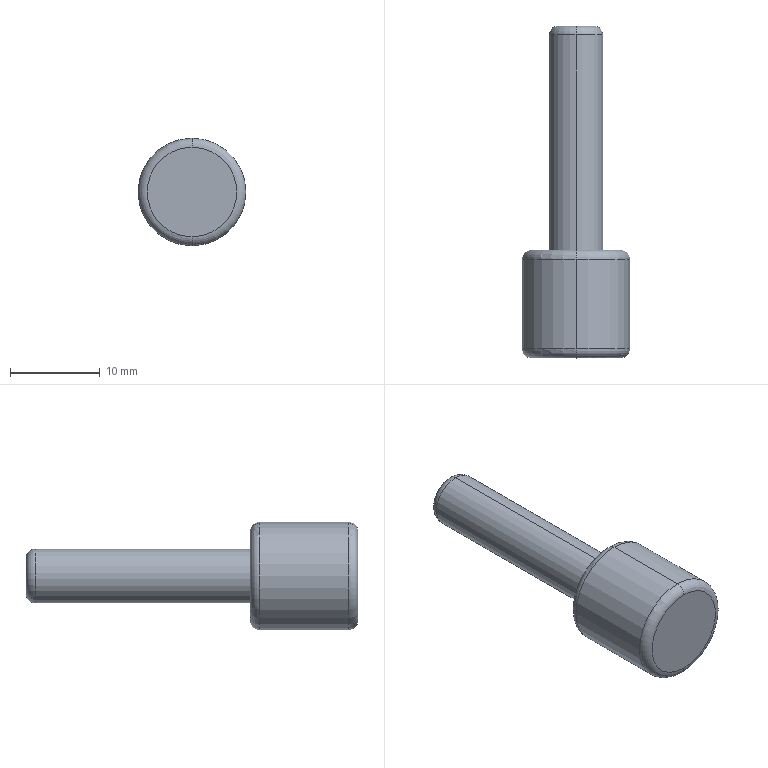Part | SolidWorks | features Extrusion 1, Fillet 1, ICE 1 | 1 solid | 13 faces | box 12 x 37 x 12 mm | volume 2045 mm3 | torus 6 | cylinder 4 | plane 3 | commonest cylinder face diameters 6 x2 12 x2
STEP:
#1=CARTESIAN_POINT('',(0.,11.,-6.));
#2=VERTEX_POINT('',#1);
#3=CARTESIAN_POINT('',(0.,11.,6.));
#4=VERTEX_POINT('',#3);
#5=CARTESIAN_POINT('',(0.,11.,0.));
#6=DIRECTION('',(0.,-1.,0.));
#7=DIRECTION('',(0.,0.,1.));
#8=AXIS2_PLACEMENT_3D('',#5,#6,#7);
#9=CIRCLE('',#8,6.);
#10=EDGE_CURVE('',#2,#4,#9,.T.);
#11=ORIENTED_EDGE('',*,*,#10,.F.);
#12=CARTESIAN_POINT('',(0.,12.,-5.));
#13=VERTEX_POINT('',#12);
#14=CARTESIAN_POINT('',(0.,11.,-5.));
#15=DIRECTION('',(1.,0.,0.));
#16=DIRECTION('',(0.,0.,-1.));
#17=AXIS2_PLACEMENT_3D('',#14,#15,#16);
#18=CIRCLE('',#17,1.);
#19=EDGE_CURVE('',#2,#13,#18,.T.);
#20=ORIENTED_EDGE('',*,*,#19,.T.);
#21=CARTESIAN_POINT('',(0.,12.,5.));
#22=VERTEX_POINT('',#21);
#23=CARTESIAN_POINT('',(0.,12.,0.));
#24=DIRECTION('',(0.,1.,0.));
#25=DIRECTION('',(0.,0.,1.));
#26=AXIS2_PLACEMENT_3D('',#23,#24,#25);
#27=CIRCLE('',#26,5.);
#28=EDGE_CURVE('',#22,#13,#27,.T.);
#29=ORIENTED_EDGE('',*,*,#28,.F.);
#30=CARTESIAN_POINT('',(0.,11.,5.));
#31=DIRECTION('',(-1.,0.,0.));
#32=DIRECTION('',(0.,0.,1.));
#33=AXIS2_PLACEMENT_3D('',#30,#31,#32);
#34=CIRCLE('',#33,1.);
#35=EDGE_CURVE('',#4,#22,#34,.T.);
#36=ORIENTED_EDGE('',*,*,#35,.F.);
#37=EDGE_LOOP('',(#11,#20,#29,#36));
#38=FACE_OUTER_BOUND('',#37,.T.);
#39=CARTESIAN_POINT('',(0.,11.,0.));
#40=DIRECTION('',(0.,1.,0.));
#41=DIRECTION('',(0.,0.,1.));
#42=AXIS2_PLACEMENT_3D('',#39,#40,#41);
#43=TOROIDAL_SURFACE('',#42,5.,1.);
#44=ADVANCED_FACE('',(#38),#43,.T.);
#45=CARTESIAN_POINT('',(0.,36.,-3.));
#46=VERTEX_POINT('',#45);
#47=CARTESIAN_POINT('',(0.,36.,3.));
#48=VERTEX_POINT('',#47);
#49=CARTESIAN_POINT('',(0.,36.,0.));
#50=DIRECTION('',(0.,-1.,0.));
#51=DIRECTION('',(0.,0.,1.));
#52=AXIS2_PLACEMENT_3D('',#49,#50,#51);
#53=CIRCLE('',#52,3.);
#54=EDGE_CURVE('',#46,#48,#53,.T.);
#55=ORIENTED_EDGE('',*,*,#54,.F.);
#56=CARTESIAN_POINT('',(0.,37.,-2.));
#57=VERTEX_POINT('',#56);
#58=CARTESIAN_POINT('',(0.,36.,-2.));
#59=DIRECTION('',(1.,0.,0.));
#60=DIRECTION('',(0.,0.,-1.));
#61=AXIS2_PLACEMENT_3D('',#58,#59,#60);
#62=CIRCLE('',#61,1.);
#63=EDGE_CURVE('',#46,#57,#62,.T.);
#64=ORIENTED_EDGE('',*,*,#63,.T.);
#65=CARTESIAN_POINT('',(0.,37.,2.));
#66=VERTEX_POINT('',#65);
#67=CARTESIAN_POINT('',(0.,37.,0.));
#68=DIRECTION('',(0.,1.,0.));
#69=DIRECTION('',(0.,0.,1.));
#70=AXIS2_PLACEMENT_3D('',#67,#68,#69);
#71=CIRCLE('',#70,2.);
#72=EDGE_CURVE('',#66,#57,#71,.T.);
#73=ORIENTED_EDGE('',*,*,#72,.F.);
#74=CARTESIAN_POINT('',(0.,36.,2.));
#75=DIRECTION('',(-1.,0.,0.));
#76=DIRECTION('',(0.,0.,1.));
#77=AXIS2_PLACEMENT_3D('',#74,#75,#76);
#78=CIRCLE('',#77,1.);
#79=EDGE_CURVE('',#48,#66,#78,.T.);
#80=ORIENTED_EDGE('',*,*,#79,.F.);
#81=EDGE_LOOP('',(#55,#64,#73,#80));
#82=FACE_OUTER_BOUND('',#81,.T.);
#83=CARTESIAN_POINT('',(0.,36.,0.));
#84=DIRECTION('',(0.,1.,0.));
#85=DIRECTION('',(0.,0.,1.));
#86=AXIS2_PLACEMENT_3D('',#83,#84,#85);
#87=TOROIDAL_SURFACE('',#86,2.,1.);
#88=ADVANCED_FACE('',(#82),#87,.T.);
#89=CARTESIAN_POINT('',(0.,0.,-5.));
#90=VERTEX_POINT('',#89);
#91=CARTESIAN_POINT('',(0.,0.,5.));
#92=VERTEX_POINT('',#91);
#93=CARTESIAN_POINT('',(0.,0.,0.));
#94=DIRECTION('',(0.,-1.,0.));
#95=DIRECTION('',(0.,0.,1.));
#96=AXIS2_PLACEMENT_3D('',#93,#94,#95);
#97=CIRCLE('',#96,5.);
#98=EDGE_CURVE('',#90,#92,#97,.T.);
#99=ORIENTED_EDGE('',*,*,#98,.F.);
#100=CARTESIAN_POINT('',(0.,1.,-6.));
#101=VERTEX_POINT('',#100);
#102=CARTESIAN_POINT('',(0.,1.,-5.));
#103=DIRECTION('',(1.,0.,0.));
#104=DIRECTION('',(0.,0.,-1.));
#105=AXIS2_PLACEMENT_3D('',#102,#103,#104);
#106=CIRCLE('',#105,1.);
#107=EDGE_CURVE('',#90,#101,#106,.T.);
#108=ORIENTED_EDGE('',*,*,#107,.T.);
#109=CARTESIAN_POINT('',(0.,1.,6.));
#110=VERTEX_POINT('',#109);
#111=CARTESIAN_POINT('',(0.,1.,0.));
#112=DIRECTION('',(0.,1.,0.));
#113=DIRECTION('',(0.,0.,1.));
#114=AXIS2_PLACEMENT_3D('',#111,#112,#113);
#115=CIRCLE('',#114,6.);
#116=EDGE_CURVE('',#110,#101,#115,.T.);
#117=ORIENTED_EDGE('',*,*,#116,.F.);
#118=CARTESIAN_POINT('',(0.,1.,5.));
#119=DIRECTION('',(-1.,0.,0.));
#120=DIRECTION('',(0.,0.,1.));
#121=AXIS2_PLACEMENT_3D('',#118,#119,#120);
#122=CIRCLE('',#121,1.);
#123=EDGE_CURVE('',#92,#110,#122,.T.);
#124=ORIENTED_EDGE('',*,*,#123,.F.);
#125=EDGE_LOOP('',(#99,#108,#117,#124));
#126=FACE_OUTER_BOUND('',#125,.T.);
#127=CARTESIAN_POINT('',(0.,1.,0.));
#128=DIRECTION('',(0.,1.,0.));
#129=DIRECTION('',(0.,0.,1.));
#130=AXIS2_PLACEMENT_3D('',#127,#128,#129);
#131=TOROIDAL_SURFACE('',#130,5.,1.);
#132=ADVANCED_FACE('',(#126),#131,.T.);
#133=ORIENTED_EDGE('',*,*,#54,.T.);
#134=CARTESIAN_POINT('',(0.,12.,3.));
#135=VERTEX_POINT('',#134);
#136=CARTESIAN_POINT('',(0.,37.,3.));
#137=DIRECTION('',(0.,-1.,0.));
#138=VECTOR('',#137,1000.);
#139=LINE('',#136,#138);
#140=EDGE_CURVE('',#48,#135,#139,.T.);
#141=ORIENTED_EDGE('',*,*,#140,.T.);
#142=CARTESIAN_POINT('',(0.,12.,-3.));
#143=VERTEX_POINT('',#142);
#144=CARTESIAN_POINT('',(0.,12.,0.));
#145=DIRECTION('',(0.,1.,0.));
#146=DIRECTION('',(0.,0.,1.));
#147=AXIS2_PLACEMENT_3D('',#144,#145,#146);
#148=CIRCLE('',#147,3.);
#149=EDGE_CURVE('',#135,#143,#148,.T.);
#150=ORIENTED_EDGE('',*,*,#149,.T.);
#151=CARTESIAN_POINT('',(0.,37.,-3.));
#152=DIRECTION('',(0.,-1.,0.));
#153=VECTOR('',#152,1000.);
#154=LINE('',#151,#153);
#155=EDGE_CURVE('',#46,#143,#154,.T.);
#156=ORIENTED_EDGE('',*,*,#155,.F.);
#157=EDGE_LOOP('',(#133,#141,#150,#156));
#158=FACE_OUTER_BOUND('',#157,.T.);
#159=CARTESIAN_POINT('',(0.,37.,0.));
#160=DIRECTION('',(0.,-1.,0.));
#161=DIRECTION('',(0.,0.,-1.));
#162=AXIS2_PLACEMENT_3D('',#159,#160,#161);
#163=CYLINDRICAL_SURFACE('',#162,3.);
#164=ADVANCED_FACE('',(#158),#163,.T.);
#165=ORIENTED_EDGE('',*,*,#10,.T.);
#166=CARTESIAN_POINT('',(0.,12.,6.));
#167=DIRECTION('',(0.,-1.,0.));
#168=VECTOR('',#167,1000.);
#169=LINE('',#166,#168);
#170=EDGE_CURVE('',#4,#110,#169,.T.);
#171=ORIENTED_EDGE('',*,*,#170,.T.);
#172=ORIENTED_EDGE('',*,*,#116,.T.);
#173=CARTESIAN_POINT('',(0.,12.,-6.));
#174=DIRECTION('',(0.,-1.,0.));
#175=VECTOR('',#174,1000.);
#176=LINE('',#173,#175);
#177=EDGE_CURVE('',#2,#101,#176,.T.);
#178=ORIENTED_EDGE('',*,*,#177,.F.);
#179=EDGE_LOOP('',(#165,#171,#172,#178));
#180=FACE_OUTER_BOUND('',#179,.T.);
#181=CARTESIAN_POINT('',(0.,12.,0.));
#182=DIRECTION('',(0.,-1.,0.));
#183=DIRECTION('',(0.,0.,-1.));
#184=AXIS2_PLACEMENT_3D('',#181,#182,#183);
#185=CYLINDRICAL_SURFACE('',#184,6.);
#186=ADVANCED_FACE('',(#180),#185,.T.);
#187=ORIENTED_EDGE('',*,*,#28,.T.);
#188=CARTESIAN_POINT('',(0.,12.,0.));
#189=DIRECTION('',(0.,1.,0.));
#190=DIRECTION('',(0.,0.,1.));
#191=AXIS2_PLACEMENT_3D('',#188,#189,#190);
#192=CIRCLE('',#191,5.);
#193=EDGE_CURVE('',#13,#22,#192,.T.);
#194=ORIENTED_EDGE('',*,*,#193,.T.);
#195=EDGE_LOOP('',(#187,#194));
#196=FACE_OUTER_BOUND('',#195,.T.);
#197=CARTESIAN_POINT('',(0.,12.,0.));
#198=DIRECTION('',(0.,1.,0.));
#199=DIRECTION('',(0.,0.,1.));
#200=AXIS2_PLACEMENT_3D('',#197,#198,#199);
#201=CIRCLE('',#200,3.);
#202=EDGE_CURVE('',#143,#135,#201,.T.);
#203=ORIENTED_EDGE('',*,*,#202,.F.);
#204=ORIENTED_EDGE('',*,*,#149,.F.);
#205=EDGE_LOOP('',(#203,#204));
#206=FACE_BOUND('',#205,.T.);
#207=CARTESIAN_POINT('',(0.,12.,0.));
#208=DIRECTION('',(0.,1.,0.));
#209=DIRECTION('',(0.,0.,1.));
#210=AXIS2_PLACEMENT_3D('',#207,#208,#209);
#211=PLANE('',#210);
#212=ADVANCED_FACE('',(#196,#206),#211,.T.);
#213=ORIENTED_EDGE('',*,*,#170,.F.);
#214=CARTESIAN_POINT('',(0.,11.,0.));
#215=DIRECTION('',(0.,-1.,0.));
#216=DIRECTION('',(0.,0.,1.));
#217=AXIS2_PLACEMENT_3D('',#214,#215,#216);
#218=CIRCLE('',#217,6.);
#219=EDGE_CURVE('',#4,#2,#218,.T.);
#220=ORIENTED_EDGE('',*,*,#219,.T.);
#221=ORIENTED_EDGE('',*,*,#177,.T.);
#222=CARTESIAN_POINT('',(0.,1.,0.));
#223=DIRECTION('',(0.,1.,0.));
#224=DIRECTION('',(0.,0.,1.));
#225=AXIS2_PLACEMENT_3D('',#222,#223,#224);
#226=CIRCLE('',#225,6.);
#227=EDGE_CURVE('',#101,#110,#226,.T.);
#228=ORIENTED_EDGE('',*,*,#227,.T.);
#229=EDGE_LOOP('',(#213,#220,#221,#228));
#230=FACE_OUTER_BOUND('',#229,.T.);
#231=CARTESIAN_POINT('',(0.,12.,0.));
#232=DIRECTION('',(0.,-1.,0.));
#233=DIRECTION('',(0.,0.,-1.));
#234=AXIS2_PLACEMENT_3D('',#231,#232,#233);
#235=CYLINDRICAL_SURFACE('',#234,6.);
#236=ADVANCED_FACE('',(#230),#235,.T.);
#237=CARTESIAN_POINT('',(0.,0.,0.));
#238=DIRECTION('',(0.,-1.,0.));
#239=DIRECTION('',(0.,0.,1.));
#240=AXIS2_PLACEMENT_3D('',#237,#238,#239);
#241=CIRCLE('',#240,5.);
#242=EDGE_CURVE('',#92,#90,#241,.T.);
#243=ORIENTED_EDGE('',*,*,#242,.T.);
#244=ORIENTED_EDGE('',*,*,#98,.T.);
#245=EDGE_LOOP('',(#243,#244));
#246=FACE_OUTER_BOUND('',#245,.T.);
#247=CARTESIAN_POINT('',(0.,0.,0.));
#248=DIRECTION('',(0.,1.,0.));
#249=DIRECTION('',(0.,0.,1.));
#250=AXIS2_PLACEMENT_3D('',#247,#248,#249);
#251=PLANE('',#250);
#252=ADVANCED_FACE('',(#246),#251,.F.);
#253=ORIENTED_EDGE('',*,*,#140,.F.);
#254=CARTESIAN_POINT('',(0.,36.,0.));
#255=DIRECTION('',(0.,-1.,0.));
#256=DIRECTION('',(0.,0.,1.));
#257=AXIS2_PLACEMENT_3D('',#254,#255,#256);
#258=CIRCLE('',#257,3.);
#259=EDGE_CURVE('',#48,#46,#258,.T.);
#260=ORIENTED_EDGE('',*,*,#259,.T.);
#261=ORIENTED_EDGE('',*,*,#155,.T.);
#262=ORIENTED_EDGE('',*,*,#202,.T.);
#263=EDGE_LOOP('',(#253,#260,#261,#262));
#264=FACE_OUTER_BOUND('',#263,.T.);
#265=CARTESIAN_POINT('',(0.,37.,0.));
#266=DIRECTION('',(0.,-1.,0.));
#267=DIRECTION('',(0.,0.,-1.));
#268=AXIS2_PLACEMENT_3D('',#265,#266,#267);
#269=CYLINDRICAL_SURFACE('',#268,3.);
#270=ADVANCED_FACE('',(#264),#269,.T.);
#271=ORIENTED_EDGE('',*,*,#72,.T.);
#272=CARTESIAN_POINT('',(0.,37.,0.));
#273=DIRECTION('',(0.,1.,0.));
#274=DIRECTION('',(0.,0.,1.));
#275=AXIS2_PLACEMENT_3D('',#272,#273,#274);
#276=CIRCLE('',#275,2.);
#277=EDGE_CURVE('',#57,#66,#276,.T.);
#278=ORIENTED_EDGE('',*,*,#277,.T.);
#279=EDGE_LOOP('',(#271,#278));
#280=FACE_OUTER_BOUND('',#279,.T.);
#281=CARTESIAN_POINT('',(0.,37.,0.));
#282=DIRECTION('',(0.,1.,0.));
#283=DIRECTION('',(0.,0.,1.));
#284=AXIS2_PLACEMENT_3D('',#281,#282,#283);
#285=PLANE('',#284);
#286=ADVANCED_FACE('',(#280),#285,.T.);
#287=ORIENTED_EDGE('',*,*,#107,.F.);
#288=ORIENTED_EDGE('',*,*,#242,.F.);
#289=ORIENTED_EDGE('',*,*,#123,.T.);
#290=ORIENTED_EDGE('',*,*,#227,.F.);
#291=EDGE_LOOP('',(#287,#288,#289,#290));
#292=FACE_OUTER_BOUND('',#291,.T.);
#293=CARTESIAN_POINT('',(0.,1.,0.));
#294=DIRECTION('',(0.,1.,0.));
#295=DIRECTION('',(0.,0.,1.));
#296=AXIS2_PLACEMENT_3D('',#293,#294,#295);
#297=TOROIDAL_SURFACE('',#296,5.,1.);
#298=ADVANCED_FACE('',(#292),#297,.T.);
#299=ORIENTED_EDGE('',*,*,#63,.F.);
#300=ORIENTED_EDGE('',*,*,#259,.F.);
#301=ORIENTED_EDGE('',*,*,#79,.T.);
#302=ORIENTED_EDGE('',*,*,#277,.F.);
#303=EDGE_LOOP('',(#299,#300,#301,#302));
#304=FACE_OUTER_BOUND('',#303,.T.);
#305=CARTESIAN_POINT('',(0.,36.,0.));
#306=DIRECTION('',(0.,1.,0.));
#307=DIRECTION('',(0.,0.,1.));
#308=AXIS2_PLACEMENT_3D('',#305,#306,#307);
#309=TOROIDAL_SURFACE('',#308,2.,1.);
#310=ADVANCED_FACE('',(#304),#309,.T.);
#311=ORIENTED_EDGE('',*,*,#19,.F.);
#312=ORIENTED_EDGE('',*,*,#219,.F.);
#313=ORIENTED_EDGE('',*,*,#35,.T.);
#314=ORIENTED_EDGE('',*,*,#193,.F.);
#315=EDGE_LOOP('',(#311,#312,#313,#314));
#316=FACE_OUTER_BOUND('',#315,.T.);
#317=CARTESIAN_POINT('',(0.,11.,0.));
#318=DIRECTION('',(0.,1.,0.));
#319=DIRECTION('',(0.,0.,1.));
#320=AXIS2_PLACEMENT_3D('',#317,#318,#319);
#321=TOROIDAL_SURFACE('',#320,5.,1.);
#322=ADVANCED_FACE('',(#316),#321,.T.);
#323=CLOSED_SHELL('',(#44,#88,#132,#164,#186,#212,#236,#252,#270,#286,#298,#310,#322));
#324=MANIFOLD_SOLID_BREP('',#323);
#325=CARTESIAN_POINT('',(0.,0.,0.));
#326=DIRECTION('',(0.,0.,1.));
#327=DIRECTION('',(1.,0.,0.));
#328=AXIS2_PLACEMENT_3D('',#325,#326,#327);
#329=(LENGTH_UNIT()NAMED_UNIT(*)SI_UNIT(.MILLI.,.METRE.));
#330=UNCERTAINTY_MEASURE_WITH_UNIT(LENGTH_MEASURE(0.00001),#329,'','');
#331=(NAMED_UNIT(*)PLANE_ANGLE_UNIT()SI_UNIT($,.RADIAN.));
#332=(NAMED_UNIT(*)SI_UNIT($,.STERADIAN.)SOLID_ANGLE_UNIT());
#333=(GEOMETRIC_REPRESENTATION_CONTEXT(3)GLOBAL_UNCERTAINTY_ASSIGNED_CONTEXT((#330))GLOBAL_UNIT_ASSIGNED_CONTEXT((#329,#331,#332))REPRESENTATION_CONTEXT('',''));
#334=ADVANCED_BREP_SHAPE_REPRESENTATION('',(#324,#328),#333);